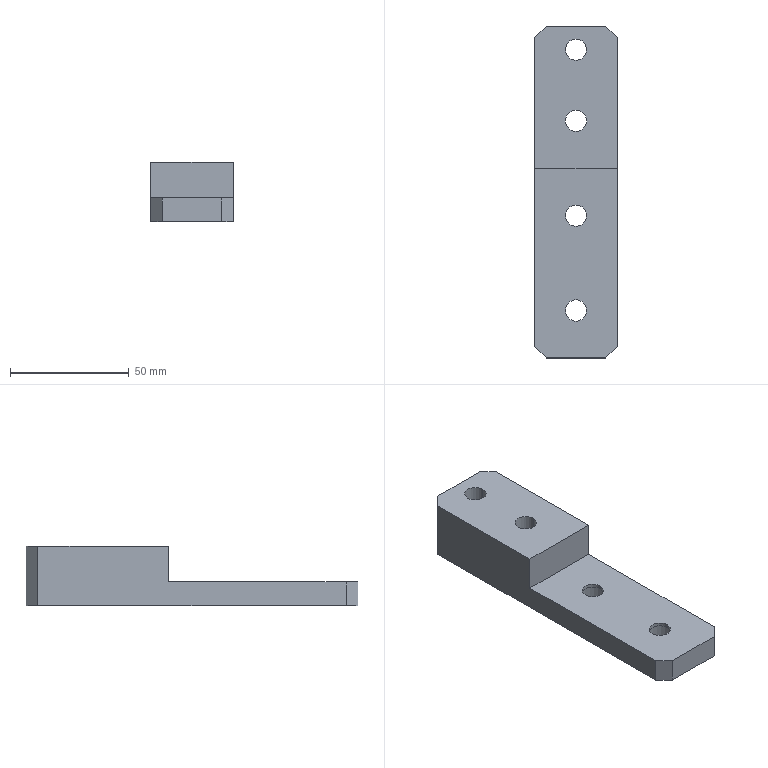Part | SolidWorks | features BaseBody 1 | 1 solid | 32 faces | box 35 x 140 x 25 mm | volume 71281 mm3 | cylinder 16 | plane 16 | commonest cylinder face diameters 9 x8 15 x8
STEP:
#1=CARTESIAN_POINT('',(7.5,-50.,8.6));
#2=VERTEX_POINT('',#1);
#3=CARTESIAN_POINT('',(-7.5,-50.,8.6));
#4=VERTEX_POINT('',#3);
#5=CARTESIAN_POINT('',(0.,-50.,8.6));
#6=DIRECTION('',(0.,0.,-1.));
#7=DIRECTION('',(-1.,0.,0.));
#8=AXIS2_PLACEMENT_3D('',#5,#6,#7);
#9=CIRCLE('',#8,7.5);
#10=EDGE_CURVE('',#2,#4,#9,.T.);
#11=ORIENTED_EDGE('',*,*,#10,.F.);
#12=CARTESIAN_POINT('',(7.5,-50.,0.));
#13=VERTEX_POINT('',#12);
#14=CARTESIAN_POINT('',(7.5,-50.,0.));
#15=DIRECTION('',(0.,0.,-1.));
#16=VECTOR('',#15,1000.);
#17=LINE('',#14,#16);
#18=EDGE_CURVE('',#2,#13,#17,.T.);
#19=ORIENTED_EDGE('',*,*,#18,.T.);
#20=CARTESIAN_POINT('',(-7.5,-50.,0.));
#21=VERTEX_POINT('',#20);
#22=CARTESIAN_POINT('',(0.,-50.,0.));
#23=DIRECTION('',(0.,0.,-1.));
#24=DIRECTION('',(-1.,0.,0.));
#25=AXIS2_PLACEMENT_3D('',#22,#23,#24);
#26=CIRCLE('',#25,7.5);
#27=EDGE_CURVE('',#13,#21,#26,.T.);
#28=ORIENTED_EDGE('',*,*,#27,.T.);
#29=CARTESIAN_POINT('',(-7.5,-50.,0.));
#30=DIRECTION('',(0.,0.,-1.));
#31=VECTOR('',#30,1000.);
#32=LINE('',#29,#31);
#33=EDGE_CURVE('',#4,#21,#32,.T.);
#34=ORIENTED_EDGE('',*,*,#33,.F.);
#35=EDGE_LOOP('',(#11,#19,#28,#34));
#36=FACE_OUTER_BOUND('',#35,.T.);
#37=CARTESIAN_POINT('',(0.,-50.,0.));
#38=DIRECTION('',(0.,0.,-1.));
#39=DIRECTION('',(-1.,0.,0.));
#40=AXIS2_PLACEMENT_3D('',#37,#38,#39);
#41=CYLINDRICAL_SURFACE('',#40,7.5);
#42=ADVANCED_FACE('',(#36),#41,.F.);
#43=CARTESIAN_POINT('',(4.5,-50.,10.));
#44=VERTEX_POINT('',#43);
#45=CARTESIAN_POINT('',(-4.5,-50.,10.));
#46=VERTEX_POINT('',#45);
#47=CARTESIAN_POINT('',(0.,-50.,10.));
#48=DIRECTION('',(0.,0.,-1.));
#49=DIRECTION('',(-1.,0.,0.));
#50=AXIS2_PLACEMENT_3D('',#47,#48,#49);
#51=CIRCLE('',#50,4.5);
#52=EDGE_CURVE('',#44,#46,#51,.T.);
#53=ORIENTED_EDGE('',*,*,#52,.F.);
#54=CARTESIAN_POINT('',(4.5,-50.,8.6));
#55=VERTEX_POINT('',#54);
#56=CARTESIAN_POINT('',(4.5,-50.,0.));
#57=DIRECTION('',(0.,0.,-1.));
#58=VECTOR('',#57,1000.);
#59=LINE('',#56,#58);
#60=EDGE_CURVE('',#44,#55,#59,.T.);
#61=ORIENTED_EDGE('',*,*,#60,.T.);
#62=CARTESIAN_POINT('',(-4.5,-50.,8.6));
#63=VERTEX_POINT('',#62);
#64=CARTESIAN_POINT('',(0.,-50.,8.6));
#65=DIRECTION('',(0.,0.,-1.));
#66=DIRECTION('',(-1.,0.,0.));
#67=AXIS2_PLACEMENT_3D('',#64,#65,#66);
#68=CIRCLE('',#67,4.5);
#69=EDGE_CURVE('',#55,#63,#68,.T.);
#70=ORIENTED_EDGE('',*,*,#69,.T.);
#71=CARTESIAN_POINT('',(-4.5,-50.,0.));
#72=DIRECTION('',(0.,0.,-1.));
#73=VECTOR('',#72,1000.);
#74=LINE('',#71,#73);
#75=EDGE_CURVE('',#46,#63,#74,.T.);
#76=ORIENTED_EDGE('',*,*,#75,.F.);
#77=EDGE_LOOP('',(#53,#61,#70,#76));
#78=FACE_OUTER_BOUND('',#77,.T.);
#79=CARTESIAN_POINT('',(0.,-50.,0.));
#80=DIRECTION('',(0.,0.,-1.));
#81=DIRECTION('',(-1.,0.,0.));
#82=AXIS2_PLACEMENT_3D('',#79,#80,#81);
#83=CYLINDRICAL_SURFACE('',#82,4.5);
#84=ADVANCED_FACE('',(#78),#83,.F.);
#85=CARTESIAN_POINT('',(7.5,-10.,8.6));
#86=VERTEX_POINT('',#85);
#87=CARTESIAN_POINT('',(-7.5,-10.,8.6));
#88=VERTEX_POINT('',#87);
#89=CARTESIAN_POINT('',(0.,-10.,8.6));
#90=DIRECTION('',(0.,0.,-1.));
#91=DIRECTION('',(-1.,0.,0.));
#92=AXIS2_PLACEMENT_3D('',#89,#90,#91);
#93=CIRCLE('',#92,7.5);
#94=EDGE_CURVE('',#86,#88,#93,.T.);
#95=ORIENTED_EDGE('',*,*,#94,.F.);
#96=CARTESIAN_POINT('',(7.5,-10.,0.));
#97=VERTEX_POINT('',#96);
#98=CARTESIAN_POINT('',(7.5,-10.,0.));
#99=DIRECTION('',(0.,0.,-1.));
#100=VECTOR('',#99,1000.);
#101=LINE('',#98,#100);
#102=EDGE_CURVE('',#86,#97,#101,.T.);
#103=ORIENTED_EDGE('',*,*,#102,.T.);
#104=CARTESIAN_POINT('',(-7.5,-10.,0.));
#105=VERTEX_POINT('',#104);
#106=CARTESIAN_POINT('',(0.,-10.,0.));
#107=DIRECTION('',(0.,0.,-1.));
#108=DIRECTION('',(-1.,0.,0.));
#109=AXIS2_PLACEMENT_3D('',#106,#107,#108);
#110=CIRCLE('',#109,7.5);
#111=EDGE_CURVE('',#97,#105,#110,.T.);
#112=ORIENTED_EDGE('',*,*,#111,.T.);
#113=CARTESIAN_POINT('',(-7.5,-10.,0.));
#114=DIRECTION('',(0.,0.,-1.));
#115=VECTOR('',#114,1000.);
#116=LINE('',#113,#115);
#117=EDGE_CURVE('',#88,#105,#116,.T.);
#118=ORIENTED_EDGE('',*,*,#117,.F.);
#119=EDGE_LOOP('',(#95,#103,#112,#118));
#120=FACE_OUTER_BOUND('',#119,.T.);
#121=CARTESIAN_POINT('',(0.,-10.,0.));
#122=DIRECTION('',(0.,0.,-1.));
#123=DIRECTION('',(-1.,0.,0.));
#124=AXIS2_PLACEMENT_3D('',#121,#122,#123);
#125=CYLINDRICAL_SURFACE('',#124,7.5);
#126=ADVANCED_FACE('',(#120),#125,.F.);
#127=CARTESIAN_POINT('',(4.5,-10.,10.));
#128=VERTEX_POINT('',#127);
#129=CARTESIAN_POINT('',(-4.5,-10.,10.));
#130=VERTEX_POINT('',#129);
#131=CARTESIAN_POINT('',(0.,-10.,10.));
#132=DIRECTION('',(0.,0.,-1.));
#133=DIRECTION('',(-1.,0.,0.));
#134=AXIS2_PLACEMENT_3D('',#131,#132,#133);
#135=CIRCLE('',#134,4.5);
#136=EDGE_CURVE('',#128,#130,#135,.T.);
#137=ORIENTED_EDGE('',*,*,#136,.F.);
#138=CARTESIAN_POINT('',(4.5,-10.,8.6));
#139=VERTEX_POINT('',#138);
#140=CARTESIAN_POINT('',(4.5,-10.,0.));
#141=DIRECTION('',(0.,0.,-1.));
#142=VECTOR('',#141,1000.);
#143=LINE('',#140,#142);
#144=EDGE_CURVE('',#128,#139,#143,.T.);
#145=ORIENTED_EDGE('',*,*,#144,.T.);
#146=CARTESIAN_POINT('',(-4.5,-10.,8.6));
#147=VERTEX_POINT('',#146);
#148=CARTESIAN_POINT('',(0.,-10.,8.6));
#149=DIRECTION('',(0.,0.,-1.));
#150=DIRECTION('',(-1.,0.,0.));
#151=AXIS2_PLACEMENT_3D('',#148,#149,#150);
#152=CIRCLE('',#151,4.5);
#153=EDGE_CURVE('',#139,#147,#152,.T.);
#154=ORIENTED_EDGE('',*,*,#153,.T.);
#155=CARTESIAN_POINT('',(-4.5,-10.,0.));
#156=DIRECTION('',(0.,0.,-1.));
#157=VECTOR('',#156,1000.);
#158=LINE('',#155,#157);
#159=EDGE_CURVE('',#130,#147,#158,.T.);
#160=ORIENTED_EDGE('',*,*,#159,.F.);
#161=EDGE_LOOP('',(#137,#145,#154,#160));
#162=FACE_OUTER_BOUND('',#161,.T.);
#163=CARTESIAN_POINT('',(0.,-10.,0.));
#164=DIRECTION('',(0.,0.,-1.));
#165=DIRECTION('',(-1.,0.,0.));
#166=AXIS2_PLACEMENT_3D('',#163,#164,#165);
#167=CYLINDRICAL_SURFACE('',#166,4.5);
#168=ADVANCED_FACE('',(#162),#167,.F.);
#169=CARTESIAN_POINT('',(7.5,60.,8.6));
#170=VERTEX_POINT('',#169);
#171=CARTESIAN_POINT('',(-7.5,60.,8.6));
#172=VERTEX_POINT('',#171);
#173=CARTESIAN_POINT('',(0.,60.,8.6));
#174=DIRECTION('',(0.,0.,-1.));
#175=DIRECTION('',(-1.,0.,0.));
#176=AXIS2_PLACEMENT_3D('',#173,#174,#175);
#177=CIRCLE('',#176,7.5);
#178=EDGE_CURVE('',#170,#172,#177,.T.);
#179=ORIENTED_EDGE('',*,*,#178,.F.);
#180=CARTESIAN_POINT('',(7.5,60.,0.));
#181=VERTEX_POINT('',#180);
#182=CARTESIAN_POINT('',(7.5,60.,0.));
#183=DIRECTION('',(0.,0.,-1.));
#184=VECTOR('',#183,1000.);
#185=LINE('',#182,#184);
#186=EDGE_CURVE('',#170,#181,#185,.T.);
#187=ORIENTED_EDGE('',*,*,#186,.T.);
#188=CARTESIAN_POINT('',(-7.5,60.,0.));
#189=VERTEX_POINT('',#188);
#190=CARTESIAN_POINT('',(0.,60.,0.));
#191=DIRECTION('',(0.,0.,-1.));
#192=DIRECTION('',(-1.,0.,0.));
#193=AXIS2_PLACEMENT_3D('',#190,#191,#192);
#194=CIRCLE('',#193,7.5);
#195=EDGE_CURVE('',#181,#189,#194,.T.);
#196=ORIENTED_EDGE('',*,*,#195,.T.);
#197=CARTESIAN_POINT('',(-7.5,60.,0.));
#198=DIRECTION('',(0.,0.,-1.));
#199=VECTOR('',#198,1000.);
#200=LINE('',#197,#199);
#201=EDGE_CURVE('',#172,#189,#200,.T.);
#202=ORIENTED_EDGE('',*,*,#201,.F.);
#203=EDGE_LOOP('',(#179,#187,#196,#202));
#204=FACE_OUTER_BOUND('',#203,.T.);
#205=CARTESIAN_POINT('',(0.,60.,0.));
#206=DIRECTION('',(0.,0.,-1.));
#207=DIRECTION('',(-1.,0.,0.));
#208=AXIS2_PLACEMENT_3D('',#205,#206,#207);
#209=CYLINDRICAL_SURFACE('',#208,7.5);
#210=ADVANCED_FACE('',(#204),#209,.F.);
#211=CARTESIAN_POINT('',(4.5,60.,25.));
#212=VERTEX_POINT('',#211);
#213=CARTESIAN_POINT('',(-4.5,60.,25.));
#214=VERTEX_POINT('',#213);
#215=CARTESIAN_POINT('',(0.,60.,25.));
#216=DIRECTION('',(0.,0.,-1.));
#217=DIRECTION('',(-1.,0.,0.));
#218=AXIS2_PLACEMENT_3D('',#215,#216,#217);
#219=CIRCLE('',#218,4.5);
#220=EDGE_CURVE('',#212,#214,#219,.T.);
#221=ORIENTED_EDGE('',*,*,#220,.F.);
#222=CARTESIAN_POINT('',(4.5,60.,8.6));
#223=VERTEX_POINT('',#222);
#224=CARTESIAN_POINT('',(4.5,60.,0.));
#225=DIRECTION('',(0.,0.,-1.));
#226=VECTOR('',#225,1000.);
#227=LINE('',#224,#226);
#228=EDGE_CURVE('',#212,#223,#227,.T.);
#229=ORIENTED_EDGE('',*,*,#228,.T.);
#230=CARTESIAN_POINT('',(-4.5,60.,8.6));
#231=VERTEX_POINT('',#230);
#232=CARTESIAN_POINT('',(0.,60.,8.6));
#233=DIRECTION('',(0.,0.,-1.));
#234=DIRECTION('',(-1.,0.,0.));
#235=AXIS2_PLACEMENT_3D('',#232,#233,#234);
#236=CIRCLE('',#235,4.5);
#237=EDGE_CURVE('',#223,#231,#236,.T.);
#238=ORIENTED_EDGE('',*,*,#237,.T.);
#239=CARTESIAN_POINT('',(-4.5,60.,0.));
#240=DIRECTION('',(0.,0.,-1.));
#241=VECTOR('',#240,1000.);
#242=LINE('',#239,#241);
#243=EDGE_CURVE('',#214,#231,#242,.T.);
#244=ORIENTED_EDGE('',*,*,#243,.F.);
#245=EDGE_LOOP('',(#221,#229,#238,#244));
#246=FACE_OUTER_BOUND('',#245,.T.);
#247=CARTESIAN_POINT('',(0.,60.,0.));
#248=DIRECTION('',(0.,0.,-1.));
#249=DIRECTION('',(-1.,0.,0.));
#250=AXIS2_PLACEMENT_3D('',#247,#248,#249);
#251=CYLINDRICAL_SURFACE('',#250,4.5);
#252=ADVANCED_FACE('',(#246),#251,.F.);
#253=CARTESIAN_POINT('',(7.5,30.,8.6));
#254=VERTEX_POINT('',#253);
#255=CARTESIAN_POINT('',(-7.5,30.,8.6));
#256=VERTEX_POINT('',#255);
#257=CARTESIAN_POINT('',(0.,30.,8.6));
#258=DIRECTION('',(0.,0.,-1.));
#259=DIRECTION('',(-1.,0.,0.));
#260=AXIS2_PLACEMENT_3D('',#257,#258,#259);
#261=CIRCLE('',#260,7.5);
#262=EDGE_CURVE('',#254,#256,#261,.T.);
#263=ORIENTED_EDGE('',*,*,#262,.F.);
#264=CARTESIAN_POINT('',(7.5,30.,0.));
#265=VERTEX_POINT('',#264);
#266=CARTESIAN_POINT('',(7.5,30.,0.));
#267=DIRECTION('',(0.,0.,-1.));
#268=VECTOR('',#267,1000.);
#269=LINE('',#266,#268);
#270=EDGE_CURVE('',#254,#265,#269,.T.);
#271=ORIENTED_EDGE('',*,*,#270,.T.);
#272=CARTESIAN_POINT('',(-7.5,30.,0.));
#273=VERTEX_POINT('',#272);
#274=CARTESIAN_POINT('',(0.,30.,0.));
#275=DIRECTION('',(0.,0.,-1.));
#276=DIRECTION('',(-1.,0.,0.));
#277=AXIS2_PLACEMENT_3D('',#274,#275,#276);
#278=CIRCLE('',#277,7.5);
#279=EDGE_CURVE('',#265,#273,#278,.T.);
#280=ORIENTED_EDGE('',*,*,#279,.T.);
#281=CARTESIAN_POINT('',(-7.5,30.,0.));
#282=DIRECTION('',(0.,0.,-1.));
#283=VECTOR('',#282,1000.);
#284=LINE('',#281,#283);
#285=EDGE_CURVE('',#256,#273,#284,.T.);
#286=ORIENTED_EDGE('',*,*,#285,.F.);
#287=EDGE_LOOP('',(#263,#271,#280,#286));
#288=FACE_OUTER_BOUND('',#287,.T.);
#289=CARTESIAN_POINT('',(0.,30.,0.));
#290=DIRECTION('',(0.,0.,-1.));
#291=DIRECTION('',(-1.,0.,0.));
#292=AXIS2_PLACEMENT_3D('',#289,#290,#291);
#293=CYLINDRICAL_SURFACE('',#292,7.5);
#294=ADVANCED_FACE('',(#288),#293,.F.);
#295=CARTESIAN_POINT('',(4.5,30.,25.));
#296=VERTEX_POINT('',#295);
#297=CARTESIAN_POINT('',(-4.5,30.,25.));
#298=VERTEX_POINT('',#297);
#299=CARTESIAN_POINT('',(0.,30.,25.));
#300=DIRECTION('',(0.,0.,-1.));
#301=DIRECTION('',(-1.,0.,0.));
#302=AXIS2_PLACEMENT_3D('',#299,#300,#301);
#303=CIRCLE('',#302,4.5);
#304=EDGE_CURVE('',#296,#298,#303,.T.);
#305=ORIENTED_EDGE('',*,*,#304,.F.);
#306=CARTESIAN_POINT('',(4.5,30.,8.6));
#307=VERTEX_POINT('',#306);
#308=CARTESIAN_POINT('',(4.5,30.,0.));
#309=DIRECTION('',(0.,0.,-1.));
#310=VECTOR('',#309,1000.);
#311=LINE('',#308,#310);
#312=EDGE_CURVE('',#296,#307,#311,.T.);
#313=ORIENTED_EDGE('',*,*,#312,.T.);
#314=CARTESIAN_POINT('',(-4.5,30.,8.6));
#315=VERTEX_POINT('',#314);
#316=CARTESIAN_POINT('',(0.,30.,8.6));
#317=DIRECTION('',(0.,0.,-1.));
#318=DIRECTION('',(-1.,0.,0.));
#319=AXIS2_PLACEMENT_3D('',#316,#317,#318);
#320=CIRCLE('',#319,4.5);
#321=EDGE_CURVE('',#307,#315,#320,.T.);
#322=ORIENTED_EDGE('',*,*,#321,.T.);
#323=CARTESIAN_POINT('',(-4.5,30.,0.));
#324=DIRECTION('',(0.,0.,-1.));
#325=VECTOR('',#324,1000.);
#326=LINE('',#323,#325);
#327=EDGE_CURVE('',#298,#315,#326,.T.);
#328=ORIENTED_EDGE('',*,*,#327,.F.);
#329=EDGE_LOOP('',(#305,#313,#322,#328));
#330=FACE_OUTER_BOUND('',#329,.T.);
#331=CARTESIAN_POINT('',(0.,30.,0.));
#332=DIRECTION('',(0.,0.,-1.));
#333=DIRECTION('',(-1.,0.,0.));
#334=AXIS2_PLACEMENT_3D('',#331,#332,#333);
#335=CYLINDRICAL_SURFACE('',#334,4.5);
#336=ADVANCED_FACE('',(#330),#335,.F.);
#337=CARTESIAN_POINT('',(-17.5,65.,0.));
#338=VERTEX_POINT('',#337);
#339=CARTESIAN_POINT('',(-17.5,-65.,0.));
#340=VERTEX_POINT('',#339);
#341=CARTESIAN_POINT('',(-17.5,70.,0.));
#342=DIRECTION('',(0.,-1.,0.));
#343=VECTOR('',#342,1000.);
#344=LINE('',#341,#343);
#345=EDGE_CURVE('',#338,#340,#344,.T.);
#346=ORIENTED_EDGE('',*,*,#345,.T.);
#347=CARTESIAN_POINT('',(-17.5,-65.,10.));
#348=VERTEX_POINT('',#347);
#349=CARTESIAN_POINT('',(-17.5,-65.,25.));
#350=DIRECTION('',(0.,0.,1.));
#351=VECTOR('',#350,1000.);
#352=LINE('',#349,#351);
#353=EDGE_CURVE('',#340,#348,#352,.T.);
#354=ORIENTED_EDGE('',*,*,#353,.T.);
#355=CARTESIAN_POINT('',(-17.5,10.,10.));
#356=VERTEX_POINT('',#355);
#357=CARTESIAN_POINT('',(-17.5,-70.,10.));
#358=DIRECTION('',(0.,-1.,0.));
#359=VECTOR('',#358,1000.);
#360=LINE('',#357,#359);
#361=EDGE_CURVE('',#356,#348,#360,.T.);
#362=ORIENTED_EDGE('',*,*,#361,.F.);
#363=CARTESIAN_POINT('',(-17.5,10.,25.));
#364=VERTEX_POINT('',#363);
#365=CARTESIAN_POINT('',(-17.5,10.,25.));
#366=DIRECTION('',(0.,0.,-1.));
#367=VECTOR('',#366,1000.);
#368=LINE('',#365,#367);
#369=EDGE_CURVE('',#364,#356,#368,.T.);
#370=ORIENTED_EDGE('',*,*,#369,.F.);
#371=CARTESIAN_POINT('',(-17.5,65.,25.));
#372=VERTEX_POINT('',#371);
#373=CARTESIAN_POINT('',(-17.5,70.,25.));
#374=DIRECTION('',(0.,-1.,0.));
#375=VECTOR('',#374,1000.);
#376=LINE('',#373,#375);
#377=EDGE_CURVE('',#372,#364,#376,.T.);
#378=ORIENTED_EDGE('',*,*,#377,.F.);
#379=CARTESIAN_POINT('',(-17.5,65.,25.));
#380=DIRECTION('',(0.,0.,-1.));
#381=VECTOR('',#380,1000.);
#382=LINE('',#379,#381);
#383=EDGE_CURVE('',#372,#338,#382,.T.);
#384=ORIENTED_EDGE('',*,*,#383,.T.);
#385=EDGE_LOOP('',(#346,#354,#362,#370,#378,#384));
#386=FACE_OUTER_BOUND('',#385,.T.);
#387=CARTESIAN_POINT('',(-17.5,70.,25.));
#388=DIRECTION('',(1.,0.,0.));
#389=DIRECTION('',(0.,1.,0.));
#390=AXIS2_PLACEMENT_3D('',#387,#388,#389);
#391=PLANE('',#390);
#392=ADVANCED_FACE('',(#386),#391,.F.);
#393=CARTESIAN_POINT('',(-12.5,-70.,0.));
#394=VERTEX_POINT('',#393);
#395=CARTESIAN_POINT('',(12.5,-70.,0.));
#396=VERTEX_POINT('',#395);
#397=CARTESIAN_POINT('',(17.5,-70.,0.));
#398=DIRECTION('',(1.,0.,0.));
#399=VECTOR('',#398,1000.);
#400=LINE('',#397,#399);
#401=EDGE_CURVE('',#394,#396,#400,.T.);
#402=ORIENTED_EDGE('',*,*,#401,.T.);
#403=CARTESIAN_POINT('',(12.5,-70.,10.));
#404=VERTEX_POINT('',#403);
#405=CARTESIAN_POINT('',(12.5,-70.,25.));
#406=DIRECTION('',(0.,0.,1.));
#407=VECTOR('',#406,1000.);
#408=LINE('',#405,#407);
#409=EDGE_CURVE('',#396,#404,#408,.T.);
#410=ORIENTED_EDGE('',*,*,#409,.T.);
#411=CARTESIAN_POINT('',(-12.5,-70.,10.));
#412=VERTEX_POINT('',#411);
#413=CARTESIAN_POINT('',(17.5,-70.,10.));
#414=DIRECTION('',(-1.,0.,0.));
#415=VECTOR('',#414,1000.);
#416=LINE('',#413,#415);
#417=EDGE_CURVE('',#404,#412,#416,.T.);
#418=ORIENTED_EDGE('',*,*,#417,.T.);
#419=CARTESIAN_POINT('',(-12.5,-70.,25.));
#420=DIRECTION('',(0.,0.,-1.));
#421=VECTOR('',#420,1000.);
#422=LINE('',#419,#421);
#423=EDGE_CURVE('',#412,#394,#422,.T.);
#424=ORIENTED_EDGE('',*,*,#423,.T.);
#425=EDGE_LOOP('',(#402,#410,#418,#424));
#426=FACE_OUTER_BOUND('',#425,.T.);
#427=CARTESIAN_POINT('',(17.5,-70.,25.));
#428=DIRECTION('',(0.,1.,0.));
#429=DIRECTION('',(0.,0.,1.));
#430=AXIS2_PLACEMENT_3D('',#427,#428,#429);
#431=PLANE('',#430);
#432=ADVANCED_FACE('',(#426),#431,.F.);
#433=CARTESIAN_POINT('',(17.5,10.,10.));
#434=VERTEX_POINT('',#433);
#435=CARTESIAN_POINT('',(17.5,-65.,10.));
#436=VERTEX_POINT('',#435);
#437=CARTESIAN_POINT('',(17.5,-70.,10.));
#438=DIRECTION('',(0.,-1.,0.));
#439=VECTOR('',#438,1000.);
#440=LINE('',#437,#439);
#441=EDGE_CURVE('',#434,#436,#440,.T.);
#442=ORIENTED_EDGE('',*,*,#441,.T.);
#443=CARTESIAN_POINT('',(17.5,-65.,0.));
#444=VERTEX_POINT('',#443);
#445=CARTESIAN_POINT('',(17.5,-65.,25.));
#446=DIRECTION('',(0.,0.,-1.));
#447=VECTOR('',#446,1000.);
#448=LINE('',#445,#447);
#449=EDGE_CURVE('',#436,#444,#448,.T.);
#450=ORIENTED_EDGE('',*,*,#449,.T.);
#451=CARTESIAN_POINT('',(17.5,65.,0.));
#452=VERTEX_POINT('',#451);
#453=CARTESIAN_POINT('',(17.5,70.,0.));
#454=DIRECTION('',(0.,1.,0.));
#455=VECTOR('',#454,1000.);
#456=LINE('',#453,#455);
#457=EDGE_CURVE('',#444,#452,#456,.T.);
#458=ORIENTED_EDGE('',*,*,#457,.T.);
#459=CARTESIAN_POINT('',(17.5,65.,25.));
#460=VERTEX_POINT('',#459);
#461=CARTESIAN_POINT('',(17.5,65.,25.));
#462=DIRECTION('',(0.,0.,1.));
#463=VECTOR('',#462,1000.);
#464=LINE('',#461,#463);
#465=EDGE_CURVE('',#452,#460,#464,.T.);
#466=ORIENTED_EDGE('',*,*,#465,.T.);
#467=CARTESIAN_POINT('',(17.5,10.,25.));
#468=VERTEX_POINT('',#467);
#469=CARTESIAN_POINT('',(17.5,70.,25.));
#470=DIRECTION('',(0.,1.,0.));
#471=VECTOR('',#470,1000.);
#472=LINE('',#469,#471);
#473=EDGE_CURVE('',#468,#460,#472,.T.);
#474=ORIENTED_EDGE('',*,*,#473,.F.);
#475=CARTESIAN_POINT('',(17.5,10.,25.));
#476=DIRECTION('',(0.,0.,-1.));
#477=VECTOR('',#476,1000.);
#478=LINE('',#475,#477);
#479=EDGE_CURVE('',#468,#434,#478,.T.);
#480=ORIENTED_EDGE('',*,*,#479,.T.);
#481=EDGE_LOOP('',(#442,#450,#458,#466,#474,#480));
#482=FACE_OUTER_BOUND('',#481,.T.);
#483=CARTESIAN_POINT('',(17.5,70.,25.));
#484=DIRECTION('',(-1.,0.,0.));
#485=DIRECTION('',(0.,-1.,0.));
#486=AXIS2_PLACEMENT_3D('',#483,#484,#485);
#487=PLANE('',#486);
#488=ADVANCED_FACE('',(#482),#487,.F.);
#489=CARTESIAN_POINT('',(12.5,70.,0.));
#490=VERTEX_POINT('',#489);
#491=CARTESIAN_POINT('',(-12.5,70.,0.));
#492=VERTEX_POINT('',#491);
#493=CARTESIAN_POINT('',(17.5,70.,0.));
#494=DIRECTION('',(-1.,0.,0.));
#495=VECTOR('',#494,1000.);
#496=LINE('',#493,#495);
#497=EDGE_CURVE('',#490,#492,#496,.T.);
#498=ORIENTED_EDGE('',*,*,#497,.T.);
#499=CARTESIAN_POINT('',(-12.5,70.,25.));
#500=VERTEX_POINT('',#499);
#501=CARTESIAN_POINT('',(-12.5,70.,25.));
#502=DIRECTION('',(0.,0.,1.));
#503=VECTOR('',#502,1000.);
#504=LINE('',#501,#503);
#505=EDGE_CURVE('',#492,#500,#504,.T.);
#506=ORIENTED_EDGE('',*,*,#505,.T.);
#507=CARTESIAN_POINT('',(12.5,70.,25.));
#508=VERTEX_POINT('',#507);
#509=CARTESIAN_POINT('',(17.5,70.,25.));
#510=DIRECTION('',(-1.,0.,0.));
#511=VECTOR('',#510,1000.);
#512=LINE('',#509,#511);
#513=EDGE_CURVE('',#508,#500,#512,.T.);
#514=ORIENTED_EDGE('',*,*,#513,.F.);
#515=CARTESIAN_POINT('',(12.5,70.,25.));
#516=DIRECTION('',(0.,0.,-1.));
#517=VECTOR('',#516,1000.);
#518=LINE('',#515,#517);
#519=EDGE_CURVE('',#508,#490,#518,.T.);
#520=ORIENTED_EDGE('',*,*,#519,.T.);
#521=EDGE_LOOP('',(#498,#506,#514,#520));
#522=FACE_OUTER_BOUND('',#521,.T.);
#523=CARTESIAN_POINT('',(17.5,70.,25.));
#524=DIRECTION('',(0.,-1.,0.));
#525=DIRECTION('',(0.,0.,-1.));
#526=AXIS2_PLACEMENT_3D('',#523,#524,#525);
#527=PLANE('',#526);
#528=ADVANCED_FACE('',(#522),#527,.F.);
#529=CARTESIAN_POINT('',(0.,60.,25.));
#530=DIRECTION('',(0.,0.,-1.));
#531=DIRECTION('',(-1.,0.,0.));
#532=AXIS2_PLACEMENT_3D('',#529,#530,#531);
#533=CIRCLE('',#532,4.5);
#534=EDGE_CURVE('',#214,#212,#533,.T.);
#535=ORIENTED_EDGE('',*,*,#534,.T.);
#536=ORIENTED_EDGE('',*,*,#220,.T.);
#537=EDGE_LOOP('',(#535,#536));
#538=FACE_BOUND('',#537,.T.);
#539=CARTESIAN_POINT('',(0.,30.,25.));
#540=DIRECTION('',(0.,0.,-1.));
#541=DIRECTION('',(-1.,0.,0.));
#542=AXIS2_PLACEMENT_3D('',#539,#540,#541);
#543=CIRCLE('',#542,4.5);
#544=EDGE_CURVE('',#298,#296,#543,.T.);
#545=ORIENTED_EDGE('',*,*,#544,.T.);
#546=ORIENTED_EDGE('',*,*,#304,.T.);
#547=EDGE_LOOP('',(#545,#546));
#548=FACE_BOUND('',#547,.T.);
#549=ORIENTED_EDGE('',*,*,#513,.T.);
#550=CARTESIAN_POINT('',(-17.5,65.,25.));
#551=DIRECTION('',(-0.7071,-0.7071,0.));
#552=VECTOR('',#551,1000.);
#553=LINE('',#550,#552);
#554=EDGE_CURVE('',#500,#372,#553,.T.);
#555=ORIENTED_EDGE('',*,*,#554,.T.);
#556=ORIENTED_EDGE('',*,*,#377,.T.);
#557=CARTESIAN_POINT('',(17.5,10.,25.));
#558=DIRECTION('',(-1.,0.,0.));
#559=VECTOR('',#558,1000.);
#560=LINE('',#557,#559);
#561=EDGE_CURVE('',#468,#364,#560,.T.);
#562=ORIENTED_EDGE('',*,*,#561,.F.);
#563=ORIENTED_EDGE('',*,*,#473,.T.);
#564=CARTESIAN_POINT('',(12.5,70.,25.));
#565=DIRECTION('',(-0.7071,0.7071,0.));
#566=VECTOR('',#565,1000.);
#567=LINE('',#564,#566);
#568=EDGE_CURVE('',#460,#508,#567,.T.);
#569=ORIENTED_EDGE('',*,*,#568,.T.);
#570=EDGE_LOOP('',(#549,#555,#556,#562,#563,#569));
#571=FACE_OUTER_BOUND('',#570,.T.);
#572=CARTESIAN_POINT('',(0.,0.,25.));
#573=DIRECTION('',(0.,0.,-1.));
#574=DIRECTION('',(-1.,0.,0.));
#575=AXIS2_PLACEMENT_3D('',#572,#573,#574);
#576=PLANE('',#575);
#577=ADVANCED_FACE('',(#538,#548,#571),#576,.F.);
#578=CARTESIAN_POINT('',(0.,-50.,0.));
#579=DIRECTION('',(0.,0.,-1.));
#580=DIRECTION('',(-1.,0.,0.));
#581=AXIS2_PLACEMENT_3D('',#578,#579,#580);
#582=CIRCLE('',#581,7.5);
#583=EDGE_CURVE('',#21,#13,#582,.T.);
#584=ORIENTED_EDGE('',*,*,#583,.F.);
#585=ORIENTED_EDGE('',*,*,#27,.F.);
#586=EDGE_LOOP('',(#584,#585));
#587=FACE_BOUND('',#586,.T.);
#588=CARTESIAN_POINT('',(0.,-10.,0.));
#589=DIRECTION('',(0.,0.,-1.));
#590=DIRECTION('',(-1.,0.,0.));
#591=AXIS2_PLACEMENT_3D('',#588,#589,#590);
#592=CIRCLE('',#591,7.5);
#593=EDGE_CURVE('',#105,#97,#592,.T.);
#594=ORIENTED_EDGE('',*,*,#593,.F.);
#595=ORIENTED_EDGE('',*,*,#111,.F.);
#596=EDGE_LOOP('',(#594,#595));
#597=FACE_BOUND('',#596,.T.);
#598=CARTESIAN_POINT('',(0.,60.,0.));
#599=DIRECTION('',(0.,0.,-1.));
#600=DIRECTION('',(-1.,0.,0.));
#601=AXIS2_PLACEMENT_3D('',#598,#599,#600);
#602=CIRCLE('',#601,7.5);
#603=EDGE_CURVE('',#189,#181,#602,.T.);
#604=ORIENTED_EDGE('',*,*,#603,.F.);
#605=ORIENTED_EDGE('',*,*,#195,.F.);
#606=EDGE_LOOP('',(#604,#605));
#607=FACE_BOUND('',#606,.T.);
#608=CARTESIAN_POINT('',(0.,30.,0.));
#609=DIRECTION('',(0.,0.,-1.));
#610=DIRECTION('',(-1.,0.,0.));
#611=AXIS2_PLACEMENT_3D('',#608,#609,#610);
#612=CIRCLE('',#611,7.5);
#613=EDGE_CURVE('',#273,#265,#612,.T.);
#614=ORIENTED_EDGE('',*,*,#613,.F.);
#615=ORIENTED_EDGE('',*,*,#279,.F.);
#616=EDGE_LOOP('',(#614,#615));
#617=FACE_BOUND('',#616,.T.);
#618=ORIENTED_EDGE('',*,*,#457,.F.);
#619=CARTESIAN_POINT('',(41.25,-41.25,0.));
#620=DIRECTION('',(-0.7071,-0.7071,0.));
#621=VECTOR('',#620,1000.);
#622=LINE('',#619,#621);
#623=EDGE_CURVE('',#444,#396,#622,.T.);
#624=ORIENTED_EDGE('',*,*,#623,.T.);
#625=ORIENTED_EDGE('',*,*,#401,.F.);
#626=CARTESIAN_POINT('',(-41.25,-41.25,0.));
#627=DIRECTION('',(-0.7071,0.7071,0.));
#628=VECTOR('',#627,1000.);
#629=LINE('',#626,#628);
#630=EDGE_CURVE('',#394,#340,#629,.T.);
#631=ORIENTED_EDGE('',*,*,#630,.T.);
#632=ORIENTED_EDGE('',*,*,#345,.F.);
#633=CARTESIAN_POINT('',(-41.25,41.25,0.));
#634=DIRECTION('',(0.7071,0.7071,0.));
#635=VECTOR('',#634,1000.);
#636=LINE('',#633,#635);
#637=EDGE_CURVE('',#338,#492,#636,.T.);
#638=ORIENTED_EDGE('',*,*,#637,.T.);
#639=ORIENTED_EDGE('',*,*,#497,.F.);
#640=CARTESIAN_POINT('',(41.25,41.25,0.));
#641=DIRECTION('',(0.7071,-0.7071,0.));
#642=VECTOR('',#641,1000.);
#643=LINE('',#640,#642);
#644=EDGE_CURVE('',#490,#452,#643,.T.);
#645=ORIENTED_EDGE('',*,*,#644,.T.);
#646=EDGE_LOOP('',(#618,#624,#625,#631,#632,#638,#639,#645));
#647=FACE_OUTER_BOUND('',#646,.T.);
#648=CARTESIAN_POINT('',(0.,0.,0.));
#649=DIRECTION('',(0.,0.,-1.));
#650=DIRECTION('',(-1.,0.,0.));
#651=AXIS2_PLACEMENT_3D('',#648,#649,#650);
#652=PLANE('',#651);
#653=ADVANCED_FACE('',(#587,#597,#607,#617,#647),#652,.T.);
#654=CARTESIAN_POINT('',(0.,-50.,10.));
#655=DIRECTION('',(0.,0.,-1.));
#656=DIRECTION('',(-1.,0.,0.));
#657=AXIS2_PLACEMENT_3D('',#654,#655,#656);
#658=CIRCLE('',#657,4.5);
#659=EDGE_CURVE('',#46,#44,#658,.T.);
#660=ORIENTED_EDGE('',*,*,#659,.T.);
#661=ORIENTED_EDGE('',*,*,#52,.T.);
#662=EDGE_LOOP('',(#660,#661));
#663=FACE_BOUND('',#662,.T.);
#664=CARTESIAN_POINT('',(0.,-10.,10.));
#665=DIRECTION('',(0.,0.,-1.));
#666=DIRECTION('',(-1.,0.,0.));
#667=AXIS2_PLACEMENT_3D('',#664,#665,#666);
#668=CIRCLE('',#667,4.5);
#669=EDGE_CURVE('',#130,#128,#668,.T.);
#670=ORIENTED_EDGE('',*,*,#669,.T.);
#671=ORIENTED_EDGE('',*,*,#136,.T.);
#672=EDGE_LOOP('',(#670,#671));
#673=FACE_BOUND('',#672,.T.);
#674=ORIENTED_EDGE('',*,*,#417,.F.);
#675=CARTESIAN_POINT('',(17.5,-65.,10.));
#676=DIRECTION('',(0.7071,0.7071,0.));
#677=VECTOR('',#676,1000.);
#678=LINE('',#675,#677);
#679=EDGE_CURVE('',#404,#436,#678,.T.);
#680=ORIENTED_EDGE('',*,*,#679,.T.);
#681=ORIENTED_EDGE('',*,*,#441,.F.);
#682=CARTESIAN_POINT('',(17.5,10.,10.));
#683=DIRECTION('',(-1.,0.,0.));
#684=VECTOR('',#683,1000.);
#685=LINE('',#682,#684);
#686=EDGE_CURVE('',#434,#356,#685,.T.);
#687=ORIENTED_EDGE('',*,*,#686,.T.);
#688=ORIENTED_EDGE('',*,*,#361,.T.);
#689=CARTESIAN_POINT('',(-12.5,-70.,10.));
#690=DIRECTION('',(0.7071,-0.7071,0.));
#691=VECTOR('',#690,1000.);
#692=LINE('',#689,#691);
#693=EDGE_CURVE('',#348,#412,#692,.T.);
#694=ORIENTED_EDGE('',*,*,#693,.T.);
#695=EDGE_LOOP('',(#674,#680,#681,#687,#688,#694));
#696=FACE_OUTER_BOUND('',#695,.T.);
#697=CARTESIAN_POINT('',(17.5,-70.,10.));
#698=DIRECTION('',(0.,0.,-1.));
#699=DIRECTION('',(-1.,0.,0.));
#700=AXIS2_PLACEMENT_3D('',#697,#698,#699);
#701=PLANE('',#700);
#702=ADVANCED_FACE('',(#663,#673,#696),#701,.F.);
#703=ORIENTED_EDGE('',*,*,#369,.T.);
#704=ORIENTED_EDGE('',*,*,#686,.F.);
#705=ORIENTED_EDGE('',*,*,#479,.F.);
#706=ORIENTED_EDGE('',*,*,#561,.T.);
#707=EDGE_LOOP('',(#703,#704,#705,#706));
#708=FACE_OUTER_BOUND('',#707,.T.);
#709=CARTESIAN_POINT('',(17.5,10.,25.));
#710=DIRECTION('',(0.,1.,0.));
#711=DIRECTION('',(0.,0.,1.));
#712=AXIS2_PLACEMENT_3D('',#709,#710,#711);
#713=PLANE('',#712);
#714=ADVANCED_FACE('',(#708),#713,.F.);
#715=ORIENTED_EDGE('',*,*,#679,.F.);
#716=ORIENTED_EDGE('',*,*,#409,.F.);
#717=ORIENTED_EDGE('',*,*,#623,.F.);
#718=ORIENTED_EDGE('',*,*,#449,.F.);
#719=EDGE_LOOP('',(#715,#716,#717,#718));
#720=FACE_OUTER_BOUND('',#719,.T.);
#721=CARTESIAN_POINT('',(17.5,-65.,25.));
#722=DIRECTION('',(-0.7071,0.7071,0.));
#723=DIRECTION('',(0.,0.,-1.));
#724=AXIS2_PLACEMENT_3D('',#721,#722,#723);
#725=PLANE('',#724);
#726=ADVANCED_FACE('',(#720),#725,.F.);
#727=ORIENTED_EDGE('',*,*,#693,.F.);
#728=ORIENTED_EDGE('',*,*,#353,.F.);
#729=ORIENTED_EDGE('',*,*,#630,.F.);
#730=ORIENTED_EDGE('',*,*,#423,.F.);
#731=EDGE_LOOP('',(#727,#728,#729,#730));
#732=FACE_OUTER_BOUND('',#731,.T.);
#733=CARTESIAN_POINT('',(-12.5,-70.,25.));
#734=DIRECTION('',(0.7071,0.7071,0.));
#735=DIRECTION('',(0.,0.,-1.));
#736=AXIS2_PLACEMENT_3D('',#733,#734,#735);
#737=PLANE('',#736);
#738=ADVANCED_FACE('',(#732),#737,.F.);
#739=ORIENTED_EDGE('',*,*,#554,.F.);
#740=ORIENTED_EDGE('',*,*,#505,.F.);
#741=ORIENTED_EDGE('',*,*,#637,.F.);
#742=ORIENTED_EDGE('',*,*,#383,.F.);
#743=EDGE_LOOP('',(#739,#740,#741,#742));
#744=FACE_OUTER_BOUND('',#743,.T.);
#745=CARTESIAN_POINT('',(-17.5,65.,25.));
#746=DIRECTION('',(0.7071,-0.7071,0.));
#747=DIRECTION('',(0.,0.,-1.));
#748=AXIS2_PLACEMENT_3D('',#745,#746,#747);
#749=PLANE('',#748);
#750=ADVANCED_FACE('',(#744),#749,.F.);
#751=ORIENTED_EDGE('',*,*,#568,.F.);
#752=ORIENTED_EDGE('',*,*,#465,.F.);
#753=ORIENTED_EDGE('',*,*,#644,.F.);
#754=ORIENTED_EDGE('',*,*,#519,.F.);
#755=EDGE_LOOP('',(#751,#752,#753,#754));
#756=FACE_OUTER_BOUND('',#755,.T.);
#757=CARTESIAN_POINT('',(12.5,70.,25.));
#758=DIRECTION('',(-0.7071,-0.7071,0.));
#759=DIRECTION('',(0.,0.,-1.));
#760=AXIS2_PLACEMENT_3D('',#757,#758,#759);
#761=PLANE('',#760);
#762=ADVANCED_FACE('',(#756),#761,.F.);
#763=ORIENTED_EDGE('',*,*,#312,.F.);
#764=ORIENTED_EDGE('',*,*,#544,.F.);
#765=ORIENTED_EDGE('',*,*,#327,.T.);
#766=CARTESIAN_POINT('',(0.,30.,8.6));
#767=DIRECTION('',(0.,0.,-1.));
#768=DIRECTION('',(-1.,0.,0.));
#769=AXIS2_PLACEMENT_3D('',#766,#767,#768);
#770=CIRCLE('',#769,4.5);
#771=EDGE_CURVE('',#315,#307,#770,.T.);
#772=ORIENTED_EDGE('',*,*,#771,.T.);
#773=EDGE_LOOP('',(#763,#764,#765,#772));
#774=FACE_OUTER_BOUND('',#773,.T.);
#775=CARTESIAN_POINT('',(0.,30.,0.));
#776=DIRECTION('',(0.,0.,-1.));
#777=DIRECTION('',(-1.,0.,0.));
#778=AXIS2_PLACEMENT_3D('',#775,#776,#777);
#779=CYLINDRICAL_SURFACE('',#778,4.5);
#780=ADVANCED_FACE('',(#774),#779,.F.);
#781=ORIENTED_EDGE('',*,*,#771,.F.);
#782=ORIENTED_EDGE('',*,*,#321,.F.);
#783=EDGE_LOOP('',(#781,#782));
#784=FACE_BOUND('',#783,.T.);
#785=CARTESIAN_POINT('',(0.,30.,8.6));
#786=DIRECTION('',(0.,0.,-1.));
#787=DIRECTION('',(-1.,0.,0.));
#788=AXIS2_PLACEMENT_3D('',#785,#786,#787);
#789=CIRCLE('',#788,7.5);
#790=EDGE_CURVE('',#256,#254,#789,.T.);
#791=ORIENTED_EDGE('',*,*,#790,.T.);
#792=ORIENTED_EDGE('',*,*,#262,.T.);
#793=EDGE_LOOP('',(#791,#792));
#794=FACE_OUTER_BOUND('',#793,.T.);
#795=CARTESIAN_POINT('',(4.5,30.,8.6));
#796=DIRECTION('',(0.,0.,1.));
#797=DIRECTION('',(1.,0.,0.));
#798=AXIS2_PLACEMENT_3D('',#795,#796,#797);
#799=PLANE('',#798);
#800=ADVANCED_FACE('',(#784,#794),#799,.F.);
#801=ORIENTED_EDGE('',*,*,#270,.F.);
#802=ORIENTED_EDGE('',*,*,#790,.F.);
#803=ORIENTED_EDGE('',*,*,#285,.T.);
#804=ORIENTED_EDGE('',*,*,#613,.T.);
#805=EDGE_LOOP('',(#801,#802,#803,#804));
#806=FACE_OUTER_BOUND('',#805,.T.);
#807=CARTESIAN_POINT('',(0.,30.,0.));
#808=DIRECTION('',(0.,0.,-1.));
#809=DIRECTION('',(-1.,0.,0.));
#810=AXIS2_PLACEMENT_3D('',#807,#808,#809);
#811=CYLINDRICAL_SURFACE('',#810,7.5);
#812=ADVANCED_FACE('',(#806),#811,.F.);
#813=ORIENTED_EDGE('',*,*,#228,.F.);
#814=ORIENTED_EDGE('',*,*,#534,.F.);
#815=ORIENTED_EDGE('',*,*,#243,.T.);
#816=CARTESIAN_POINT('',(0.,60.,8.6));
#817=DIRECTION('',(0.,0.,-1.));
#818=DIRECTION('',(-1.,0.,0.));
#819=AXIS2_PLACEMENT_3D('',#816,#817,#818);
#820=CIRCLE('',#819,4.5);
#821=EDGE_CURVE('',#231,#223,#820,.T.);
#822=ORIENTED_EDGE('',*,*,#821,.T.);
#823=EDGE_LOOP('',(#813,#814,#815,#822));
#824=FACE_OUTER_BOUND('',#823,.T.);
#825=CARTESIAN_POINT('',(0.,60.,0.));
#826=DIRECTION('',(0.,0.,-1.));
#827=DIRECTION('',(-1.,0.,0.));
#828=AXIS2_PLACEMENT_3D('',#825,#826,#827);
#829=CYLINDRICAL_SURFACE('',#828,4.5);
#830=ADVANCED_FACE('',(#824),#829,.F.);
#831=ORIENTED_EDGE('',*,*,#821,.F.);
#832=ORIENTED_EDGE('',*,*,#237,.F.);
#833=EDGE_LOOP('',(#831,#832));
#834=FACE_BOUND('',#833,.T.);
#835=CARTESIAN_POINT('',(0.,60.,8.6));
#836=DIRECTION('',(0.,0.,-1.));
#837=DIRECTION('',(-1.,0.,0.));
#838=AXIS2_PLACEMENT_3D('',#835,#836,#837);
#839=CIRCLE('',#838,7.5);
#840=EDGE_CURVE('',#172,#170,#839,.T.);
#841=ORIENTED_EDGE('',*,*,#840,.T.);
#842=ORIENTED_EDGE('',*,*,#178,.T.);
#843=EDGE_LOOP('',(#841,#842));
#844=FACE_OUTER_BOUND('',#843,.T.);
#845=CARTESIAN_POINT('',(4.5,60.,8.6));
#846=DIRECTION('',(0.,0.,1.));
#847=DIRECTION('',(1.,0.,0.));
#848=AXIS2_PLACEMENT_3D('',#845,#846,#847);
#849=PLANE('',#848);
#850=ADVANCED_FACE('',(#834,#844),#849,.F.);
#851=ORIENTED_EDGE('',*,*,#186,.F.);
#852=ORIENTED_EDGE('',*,*,#840,.F.);
#853=ORIENTED_EDGE('',*,*,#201,.T.);
#854=ORIENTED_EDGE('',*,*,#603,.T.);
#855=EDGE_LOOP('',(#851,#852,#853,#854));
#856=FACE_OUTER_BOUND('',#855,.T.);
#857=CARTESIAN_POINT('',(0.,60.,0.));
#858=DIRECTION('',(0.,0.,-1.));
#859=DIRECTION('',(-1.,0.,0.));
#860=AXIS2_PLACEMENT_3D('',#857,#858,#859);
#861=CYLINDRICAL_SURFACE('',#860,7.5);
#862=ADVANCED_FACE('',(#856),#861,.F.);
#863=ORIENTED_EDGE('',*,*,#144,.F.);
#864=ORIENTED_EDGE('',*,*,#669,.F.);
#865=ORIENTED_EDGE('',*,*,#159,.T.);
#866=CARTESIAN_POINT('',(0.,-10.,8.6));
#867=DIRECTION('',(0.,0.,-1.));
#868=DIRECTION('',(-1.,0.,0.));
#869=AXIS2_PLACEMENT_3D('',#866,#867,#868);
#870=CIRCLE('',#869,4.5);
#871=EDGE_CURVE('',#147,#139,#870,.T.);
#872=ORIENTED_EDGE('',*,*,#871,.T.);
#873=EDGE_LOOP('',(#863,#864,#865,#872));
#874=FACE_OUTER_BOUND('',#873,.T.);
#875=CARTESIAN_POINT('',(0.,-10.,0.));
#876=DIRECTION('',(0.,0.,-1.));
#877=DIRECTION('',(-1.,0.,0.));
#878=AXIS2_PLACEMENT_3D('',#875,#876,#877);
#879=CYLINDRICAL_SURFACE('',#878,4.5);
#880=ADVANCED_FACE('',(#874),#879,.F.);
#881=ORIENTED_EDGE('',*,*,#871,.F.);
#882=ORIENTED_EDGE('',*,*,#153,.F.);
#883=EDGE_LOOP('',(#881,#882));
#884=FACE_BOUND('',#883,.T.);
#885=CARTESIAN_POINT('',(0.,-10.,8.6));
#886=DIRECTION('',(0.,0.,-1.));
#887=DIRECTION('',(-1.,0.,0.));
#888=AXIS2_PLACEMENT_3D('',#885,#886,#887);
#889=CIRCLE('',#888,7.5);
#890=EDGE_CURVE('',#88,#86,#889,.T.);
#891=ORIENTED_EDGE('',*,*,#890,.T.);
#892=ORIENTED_EDGE('',*,*,#94,.T.);
#893=EDGE_LOOP('',(#891,#892));
#894=FACE_OUTER_BOUND('',#893,.T.);
#895=CARTESIAN_POINT('',(4.5,-10.,8.6));
#896=DIRECTION('',(0.,0.,1.));
#897=DIRECTION('',(1.,0.,0.));
#898=AXIS2_PLACEMENT_3D('',#895,#896,#897);
#899=PLANE('',#898);
#900=ADVANCED_FACE('',(#884,#894),#899,.F.);
#901=ORIENTED_EDGE('',*,*,#102,.F.);
#902=ORIENTED_EDGE('',*,*,#890,.F.);
#903=ORIENTED_EDGE('',*,*,#117,.T.);
#904=ORIENTED_EDGE('',*,*,#593,.T.);
#905=EDGE_LOOP('',(#901,#902,#903,#904));
#906=FACE_OUTER_BOUND('',#905,.T.);
#907=CARTESIAN_POINT('',(0.,-10.,0.));
#908=DIRECTION('',(0.,0.,-1.));
#909=DIRECTION('',(-1.,0.,0.));
#910=AXIS2_PLACEMENT_3D('',#907,#908,#909);
#911=CYLINDRICAL_SURFACE('',#910,7.5);
#912=ADVANCED_FACE('',(#906),#911,.F.);
#913=ORIENTED_EDGE('',*,*,#60,.F.);
#914=ORIENTED_EDGE('',*,*,#659,.F.);
#915=ORIENTED_EDGE('',*,*,#75,.T.);
#916=CARTESIAN_POINT('',(0.,-50.,8.6));
#917=DIRECTION('',(0.,0.,-1.));
#918=DIRECTION('',(-1.,0.,0.));
#919=AXIS2_PLACEMENT_3D('',#916,#917,#918);
#920=CIRCLE('',#919,4.5);
#921=EDGE_CURVE('',#63,#55,#920,.T.);
#922=ORIENTED_EDGE('',*,*,#921,.T.);
#923=EDGE_LOOP('',(#913,#914,#915,#922));
#924=FACE_OUTER_BOUND('',#923,.T.);
#925=CARTESIAN_POINT('',(0.,-50.,0.));
#926=DIRECTION('',(0.,0.,-1.));
#927=DIRECTION('',(-1.,0.,0.));
#928=AXIS2_PLACEMENT_3D('',#925,#926,#927);
#929=CYLINDRICAL_SURFACE('',#928,4.5);
#930=ADVANCED_FACE('',(#924),#929,.F.);
#931=ORIENTED_EDGE('',*,*,#921,.F.);
#932=ORIENTED_EDGE('',*,*,#69,.F.);
#933=EDGE_LOOP('',(#931,#932));
#934=FACE_BOUND('',#933,.T.);
#935=CARTESIAN_POINT('',(0.,-50.,8.6));
#936=DIRECTION('',(0.,0.,-1.));
#937=DIRECTION('',(-1.,0.,0.));
#938=AXIS2_PLACEMENT_3D('',#935,#936,#937);
#939=CIRCLE('',#938,7.5);
#940=EDGE_CURVE('',#4,#2,#939,.T.);
#941=ORIENTED_EDGE('',*,*,#940,.T.);
#942=ORIENTED_EDGE('',*,*,#10,.T.);
#943=EDGE_LOOP('',(#941,#942));
#944=FACE_OUTER_BOUND('',#943,.T.);
#945=CARTESIAN_POINT('',(4.5,-50.,8.6));
#946=DIRECTION('',(0.,0.,1.));
#947=DIRECTION('',(1.,0.,0.));
#948=AXIS2_PLACEMENT_3D('',#945,#946,#947);
#949=PLANE('',#948);
#950=ADVANCED_FACE('',(#934,#944),#949,.F.);
#951=ORIENTED_EDGE('',*,*,#18,.F.);
#952=ORIENTED_EDGE('',*,*,#940,.F.);
#953=ORIENTED_EDGE('',*,*,#33,.T.);
#954=ORIENTED_EDGE('',*,*,#583,.T.);
#955=EDGE_LOOP('',(#951,#952,#953,#954));
#956=FACE_OUTER_BOUND('',#955,.T.);
#957=CARTESIAN_POINT('',(0.,-50.,0.));
#958=DIRECTION('',(0.,0.,-1.));
#959=DIRECTION('',(-1.,0.,0.));
#960=AXIS2_PLACEMENT_3D('',#957,#958,#959);
#961=CYLINDRICAL_SURFACE('',#960,7.5);
#962=ADVANCED_FACE('',(#956),#961,.F.);
#963=CLOSED_SHELL('',(#42,#84,#126,#168,#210,#252,#294,#336,#392,#432,#488,#528,#577,#653,#702,#714,#726,#738,#750,#762,#780,#800,#812,#830,#850,#862,#880,#900,#912,#930,#950,#962));
#964=MANIFOLD_SOLID_BREP('',#963);
#965=CARTESIAN_POINT('',(0.,0.,0.));
#966=DIRECTION('',(0.,0.,1.));
#967=DIRECTION('',(1.,0.,0.));
#968=AXIS2_PLACEMENT_3D('',#965,#966,#967);
#969=(LENGTH_UNIT()NAMED_UNIT(*)SI_UNIT(.MILLI.,.METRE.));
#970=UNCERTAINTY_MEASURE_WITH_UNIT(LENGTH_MEASURE(0.00001),#969,'','');
#971=(NAMED_UNIT(*)PLANE_ANGLE_UNIT()SI_UNIT($,.RADIAN.));
#972=(NAMED_UNIT(*)SI_UNIT($,.STERADIAN.)SOLID_ANGLE_UNIT());
#973=(GEOMETRIC_REPRESENTATION_CONTEXT(3)GLOBAL_UNCERTAINTY_ASSIGNED_CONTEXT((#970))GLOBAL_UNIT_ASSIGNED_CONTEXT((#969,#971,#972))REPRESENTATION_CONTEXT('',''));
#974=ADVANCED_BREP_SHAPE_REPRESENTATION('',(#964,#968),#973);